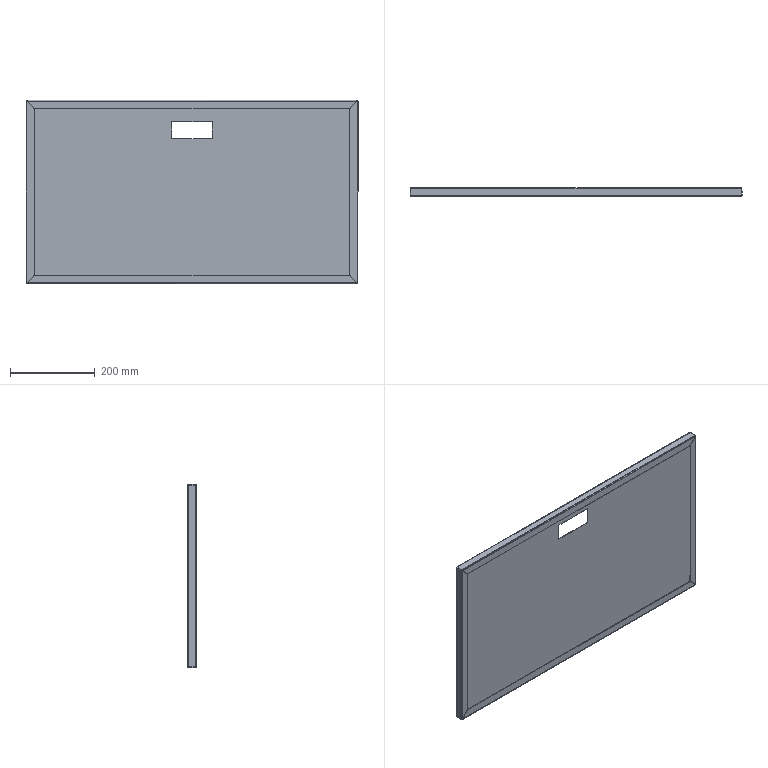Part | SolidWorks | features EdgeFlange 2, FlatPattern 1, ICE 1, SMBaseFlange 1, SheetMetal 1 | 1 solid | 74 faces | box 782 x 20 x 432 mm | volume 503943 mm3 | plane 42 | spline 16 | cylinder 16 | commonest cylinder face diameters 2 x8 4.4 x8